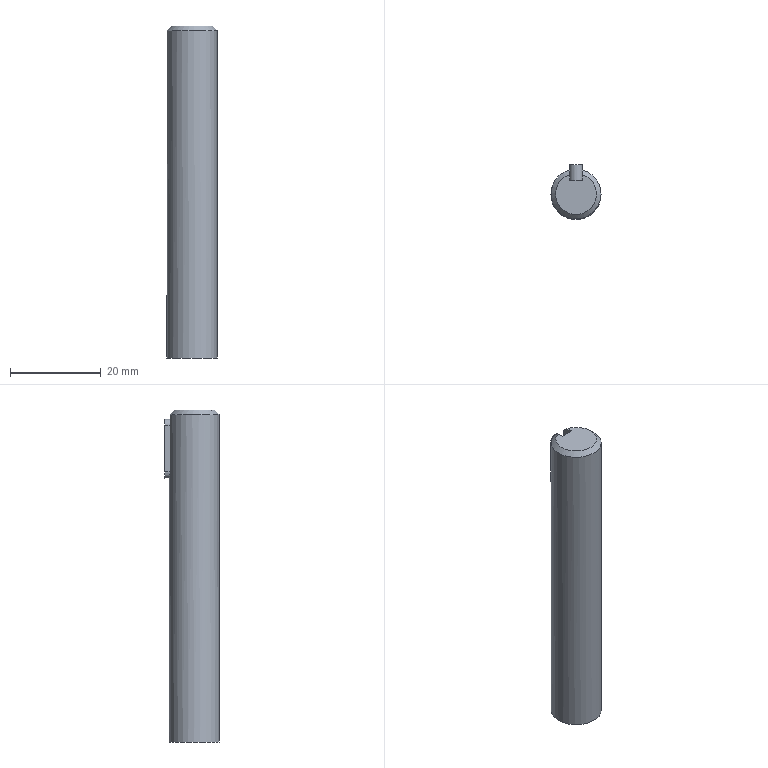Part | NX | features DATUM_CSYS 3, EXTRUDE 3, SKETCH 3, BLEND 2, BREP 1, CHAMFER 1 | 2 solids | 14 faces | box 11 x 12 x 73 mm | volume 6944 mm3 | plane 9 | cylinder 4 | cone 1 | commonest cylinder face diameters 2.8 x3 11 x1
STEP:
#1=CARTESIAN_POINT('',(-1.4,3.,69.6));
#2=VERTEX_POINT('',#1);
#3=CARTESIAN_POINT('',(-1.4,3.,59.4));
#4=VERTEX_POINT('',#3);
#5=CARTESIAN_POINT('',(-1.4,3.,71.));
#6=DIRECTION('',(0.,0.,-1.));
#7=VECTOR('',#6,1000.);
#8=LINE('',#5,#7);
#9=EDGE_CURVE('',#2,#4,#8,.T.);
#10=ORIENTED_EDGE('',*,*,#9,.F.);
#11=CARTESIAN_POINT('',(-1.4,6.5,69.6));
#12=VERTEX_POINT('',#11);
#13=CARTESIAN_POINT('',(-1.4,6.5,69.6));
#14=DIRECTION('',(0.,-1.,0.));
#15=VECTOR('',#14,1000.);
#16=LINE('',#13,#15);
#17=EDGE_CURVE('',#2,#12,#16,.F.);
#18=ORIENTED_EDGE('',*,*,#17,.T.);
#19=CARTESIAN_POINT('',(-1.4,6.5,59.4));
#20=VERTEX_POINT('',#19);
#21=CARTESIAN_POINT('',(-1.4,6.5,71.));
#22=DIRECTION('',(0.,0.,-1.));
#23=VECTOR('',#22,1000.);
#24=LINE('',#21,#23);
#25=EDGE_CURVE('',#12,#20,#24,.T.);
#26=ORIENTED_EDGE('',*,*,#25,.T.);
#27=CARTESIAN_POINT('',(-1.4,6.5,59.4));
#28=DIRECTION('',(0.,-1.,0.));
#29=VECTOR('',#28,1000.);
#30=LINE('',#27,#29);
#31=EDGE_CURVE('',#20,#4,#30,.T.);
#32=ORIENTED_EDGE('',*,*,#31,.T.);
#33=EDGE_LOOP('',(#10,#18,#26,#32));
#34=FACE_BOUND('',#33,.T.);
#35=CARTESIAN_POINT('',(-1.4,6.5,71.));
#36=DIRECTION('',(1.,0.,0.));
#37=DIRECTION('',(0.,1.,0.));
#38=AXIS2_PLACEMENT_3D('',#35,#36,#37);
#39=PLANE('',#38);
#40=ADVANCED_FACE('',(#34),#39,.F.);
#41=CARTESIAN_POINT('',(1.4,3.,69.6));
#42=VERTEX_POINT('',#41);
#43=CARTESIAN_POINT('',(0.,3.,69.6));
#44=DIRECTION('',(0.,1.,0.));
#45=DIRECTION('',(-1.,0.,0.));
#46=AXIS2_PLACEMENT_3D('',#43,#44,#45);
#47=CIRCLE('',#46,1.4);
#48=EDGE_CURVE('',#42,#2,#47,.F.);
#49=ORIENTED_EDGE('',*,*,#48,.T.);
#50=ORIENTED_EDGE('',*,*,#9,.T.);
#51=CARTESIAN_POINT('',(1.4,3.,59.4));
#52=VERTEX_POINT('',#51);
#53=CARTESIAN_POINT('',(0.,3.,59.4));
#54=DIRECTION('',(0.,1.,0.));
#55=DIRECTION('',(-1.,0.,0.));
#56=AXIS2_PLACEMENT_3D('',#53,#54,#55);
#57=CIRCLE('',#56,1.4);
#58=EDGE_CURVE('',#4,#52,#57,.F.);
#59=ORIENTED_EDGE('',*,*,#58,.T.);
#60=CARTESIAN_POINT('',(1.4,3.,71.));
#61=DIRECTION('',(0.,0.,-1.));
#62=VECTOR('',#61,1000.);
#63=LINE('',#60,#62);
#64=EDGE_CURVE('',#42,#52,#63,.T.);
#65=ORIENTED_EDGE('',*,*,#64,.F.);
#66=EDGE_LOOP('',(#49,#50,#59,#65));
#67=FACE_BOUND('',#66,.T.);
#68=CARTESIAN_POINT('',(-1.4,3.,71.));
#69=DIRECTION('',(0.,1.,0.));
#70=DIRECTION('',(-1.,0.,0.));
#71=AXIS2_PLACEMENT_3D('',#68,#69,#70);
#72=PLANE('',#71);
#73=ADVANCED_FACE('',(#67),#72,.F.);
#74=CARTESIAN_POINT('',(1.4,6.5,69.6));
#75=VERTEX_POINT('',#74);
#76=CARTESIAN_POINT('',(1.4,6.5,59.4));
#77=VERTEX_POINT('',#76);
#78=CARTESIAN_POINT('',(1.4,6.5,71.));
#79=DIRECTION('',(0.,0.,-1.));
#80=VECTOR('',#79,1000.);
#81=LINE('',#78,#80);
#82=EDGE_CURVE('',#75,#77,#81,.T.);
#83=ORIENTED_EDGE('',*,*,#82,.F.);
#84=CARTESIAN_POINT('',(1.4,3.,69.6));
#85=DIRECTION('',(0.,1.,0.));
#86=VECTOR('',#85,1000.);
#87=LINE('',#84,#86);
#88=EDGE_CURVE('',#75,#42,#87,.F.);
#89=ORIENTED_EDGE('',*,*,#88,.T.);
#90=ORIENTED_EDGE('',*,*,#64,.T.);
#91=CARTESIAN_POINT('',(1.4,3.,59.4));
#92=DIRECTION('',(0.,1.,0.));
#93=VECTOR('',#92,1000.);
#94=LINE('',#91,#93);
#95=EDGE_CURVE('',#52,#77,#94,.T.);
#96=ORIENTED_EDGE('',*,*,#95,.T.);
#97=EDGE_LOOP('',(#83,#89,#90,#96));
#98=FACE_BOUND('',#97,.T.);
#99=CARTESIAN_POINT('',(1.4,3.,71.));
#100=DIRECTION('',(-1.,0.,0.));
#101=DIRECTION('',(0.,-1.,0.));
#102=AXIS2_PLACEMENT_3D('',#99,#100,#101);
#103=PLANE('',#102);
#104=ADVANCED_FACE('',(#98),#103,.F.);
#105=ORIENTED_EDGE('',*,*,#25,.F.);
#106=CARTESIAN_POINT('',(0.,6.5,69.6));
#107=DIRECTION('',(0.,-1.,0.));
#108=DIRECTION('',(0.,0.,-1.));
#109=AXIS2_PLACEMENT_3D('',#106,#107,#108);
#110=CIRCLE('',#109,1.4);
#111=EDGE_CURVE('',#12,#75,#110,.F.);
#112=ORIENTED_EDGE('',*,*,#111,.T.);
#113=ORIENTED_EDGE('',*,*,#82,.T.);
#114=CARTESIAN_POINT('',(0.,6.5,59.4));
#115=DIRECTION('',(0.,-1.,0.));
#116=DIRECTION('',(0.,0.,-1.));
#117=AXIS2_PLACEMENT_3D('',#114,#115,#116);
#118=CIRCLE('',#117,1.4);
#119=EDGE_CURVE('',#77,#20,#118,.F.);
#120=ORIENTED_EDGE('',*,*,#119,.T.);
#121=EDGE_LOOP('',(#105,#112,#113,#120));
#122=FACE_BOUND('',#121,.T.);
#123=CARTESIAN_POINT('',(1.4,6.5,71.));
#124=DIRECTION('',(0.,-1.,0.));
#125=DIRECTION('',(0.,0.,-1.));
#126=AXIS2_PLACEMENT_3D('',#123,#124,#125);
#127=PLANE('',#126);
#128=ADVANCED_FACE('',(#122),#127,.F.);
#129=ORIENTED_EDGE('',*,*,#88,.F.);
#130=ORIENTED_EDGE('',*,*,#111,.F.);
#131=ORIENTED_EDGE('',*,*,#17,.F.);
#132=ORIENTED_EDGE('',*,*,#48,.F.);
#133=EDGE_LOOP('',(#129,#130,#131,#132));
#134=FACE_BOUND('',#133,.T.);
#135=CARTESIAN_POINT('',(0.,0.,69.6));
#136=DIRECTION('',(0.,-1.,0.));
#137=DIRECTION('',(1.,0.,0.));
#138=AXIS2_PLACEMENT_3D('',#135,#136,#137);
#139=CYLINDRICAL_SURFACE('',#138,1.4);
#140=ADVANCED_FACE('',(#134),#139,.T.);
#141=ORIENTED_EDGE('',*,*,#58,.F.);
#142=ORIENTED_EDGE('',*,*,#31,.F.);
#143=ORIENTED_EDGE('',*,*,#119,.F.);
#144=ORIENTED_EDGE('',*,*,#95,.F.);
#145=EDGE_LOOP('',(#141,#142,#143,#144));
#146=FACE_BOUND('',#145,.T.);
#147=CARTESIAN_POINT('',(0.,3.,59.4));
#148=DIRECTION('',(0.,1.,0.));
#149=DIRECTION('',(-1.,0.,0.));
#150=AXIS2_PLACEMENT_3D('',#147,#148,#149);
#151=CYLINDRICAL_SURFACE('',#150,1.4);
#152=ADVANCED_FACE('',(#146),#151,.T.);
#153=CLOSED_SHELL('',(#40,#73,#104,#128,#140,#152));
#154=MANIFOLD_SOLID_BREP('',#153);
#155=CARTESIAN_POINT('',(-1.4,4.277,73.));
#156=VERTEX_POINT('',#155);
#157=CARTESIAN_POINT('',(-1.4,3.,73.));
#158=VERTEX_POINT('',#157);
#159=CARTESIAN_POINT('',(-1.4,0.,73.));
#160=DIRECTION('',(0.,-1.,0.));
#161=VECTOR('',#160,1000.);
#162=LINE('',#159,#161);
#163=EDGE_CURVE('',#156,#158,#162,.T.);
#164=ORIENTED_EDGE('',*,*,#163,.F.);
#165=CARTESIAN_POINT('',(1.4,4.277,73.));
#166=VERTEX_POINT('',#165);
#167=CARTESIAN_POINT('',(0.,0.,73.));
#168=DIRECTION('',(0.,0.,1.));
#169=DIRECTION('',(1.,0.,0.));
#170=AXIS2_PLACEMENT_3D('',#167,#168,#169);
#171=CIRCLE('',#170,4.5);
#172=EDGE_CURVE('',#156,#166,#171,.T.);
#173=ORIENTED_EDGE('',*,*,#172,.T.);
#174=CARTESIAN_POINT('',(1.4,3.,73.));
#175=VERTEX_POINT('',#174);
#176=CARTESIAN_POINT('',(1.4,0.,73.));
#177=DIRECTION('',(0.,1.,0.));
#178=VECTOR('',#177,1000.);
#179=LINE('',#176,#178);
#180=EDGE_CURVE('',#175,#166,#179,.T.);
#181=ORIENTED_EDGE('',*,*,#180,.F.);
#182=CARTESIAN_POINT('',(0.,3.,73.));
#183=DIRECTION('',(-1.,0.,0.));
#184=VECTOR('',#183,1000.);
#185=LINE('',#182,#184);
#186=EDGE_CURVE('',#175,#158,#185,.T.);
#187=ORIENTED_EDGE('',*,*,#186,.T.);
#188=EDGE_LOOP('',(#164,#173,#181,#187));
#189=FACE_BOUND('',#188,.T.);
#190=CARTESIAN_POINT('',(0.,0.,73.));
#191=DIRECTION('',(0.,0.,1.));
#192=DIRECTION('',(1.,0.,0.));
#193=AXIS2_PLACEMENT_3D('',#190,#191,#192);
#194=PLANE('',#193);
#195=ADVANCED_FACE('',(#189),#194,.T.);
#196=CARTESIAN_POINT('',(1.4,5.319,72.));
#197=VERTEX_POINT('',#196);
#198=CARTESIAN_POINT('',(1.4,5.319,59.4));
#199=VERTEX_POINT('',#198);
#200=CARTESIAN_POINT('',(1.4,5.319,0.));
#201=DIRECTION('',(0.,0.,-1.));
#202=VECTOR('',#201,1000.);
#203=LINE('',#200,#202);
#204=EDGE_CURVE('',#197,#199,#203,.T.);
#205=ORIENTED_EDGE('',*,*,#204,.F.);
#206=CARTESIAN_POINT('',(-1.4,5.319,72.));
#207=VERTEX_POINT('',#206);
#208=CARTESIAN_POINT('',(0.,0.,72.));
#209=DIRECTION('',(0.,0.,1.));
#210=DIRECTION('',(1.,0.,0.));
#211=AXIS2_PLACEMENT_3D('',#208,#209,#210);
#212=CIRCLE('',#211,5.5);
#213=EDGE_CURVE('',#197,#207,#212,.F.);
#214=ORIENTED_EDGE('',*,*,#213,.T.);
#215=CARTESIAN_POINT('',(-1.4,5.319,59.4));
#216=VERTEX_POINT('',#215);
#217=CARTESIAN_POINT('',(-1.4,5.319,0.));
#218=DIRECTION('',(0.,0.,-1.));
#219=VECTOR('',#218,1000.);
#220=LINE('',#217,#219);
#221=EDGE_CURVE('',#216,#207,#220,.F.);
#222=ORIENTED_EDGE('',*,*,#221,.F.);
#223=CARTESIAN_POINT('',(-1.4,5.319,59.4));
#224=CARTESIAN_POINT('',(-1.4,5.319,59.029));
#225=CARTESIAN_POINT('',(-1.098,5.411,58.306));
#226=CARTESIAN_POINT('',(0.000296,5.545,57.847));
#227=CARTESIAN_POINT('',(1.097,5.411,58.305));
#228=CARTESIAN_POINT('',(1.4,5.319,59.029));
#229=CARTESIAN_POINT('',(1.4,5.319,59.4));
#230=B_SPLINE_CURVE_WITH_KNOTS('',3,(#223,#224,#225,#226,#227,#228,#229),.UNSPECIFIED.,.F.,.F.,(4,1,1,1,4),(0.,0.001098,0.002196,0.003294,0.004392),.UNSPECIFIED.);
#231=EDGE_CURVE('',#216,#199,#230,.T.);
#232=ORIENTED_EDGE('',*,*,#231,.T.);
#233=EDGE_LOOP('',(#205,#214,#222,#232));
#234=FACE_BOUND('',#233,.T.);
#235=CARTESIAN_POINT('',(-5.5,0.,0.));
#236=VERTEX_POINT('',#235);
#237=CARTESIAN_POINT('',(-5.5,0.,4.));
#238=VERTEX_POINT('',#237);
#239=CARTESIAN_POINT('',(-5.5,0.,0.));
#240=DIRECTION('',(0.,0.,-1.));
#241=VECTOR('',#240,1000.);
#242=LINE('',#239,#241);
#243=EDGE_CURVE('',#236,#238,#242,.F.);
#244=ORIENTED_EDGE('',*,*,#243,.T.);
#245=ORIENTED_EDGE('',*,*,#243,.F.);
#246=CARTESIAN_POINT('',(5.5,0.,0.));
#247=VERTEX_POINT('',#246);
#248=CARTESIAN_POINT('',(0.,0.,0.));
#249=DIRECTION('',(0.,0.,-1.));
#250=DIRECTION('',(-1.,0.,0.));
#251=AXIS2_PLACEMENT_3D('',#248,#249,#250);
#252=CIRCLE('',#251,5.5);
#253=EDGE_CURVE('',#247,#236,#252,.T.);
#254=ORIENTED_EDGE('',*,*,#253,.F.);
#255=CARTESIAN_POINT('',(5.5,0.,4.));
#256=VERTEX_POINT('',#255);
#257=CARTESIAN_POINT('',(5.5,0.,0.));
#258=DIRECTION('',(0.,0.,-1.));
#259=VECTOR('',#258,1000.);
#260=LINE('',#257,#259);
#261=EDGE_CURVE('',#247,#256,#260,.F.);
#262=ORIENTED_EDGE('',*,*,#261,.T.);
#263=ORIENTED_EDGE('',*,*,#261,.F.);
#264=CARTESIAN_POINT('',(0.,0.,0.));
#265=DIRECTION('',(0.,0.,-1.));
#266=DIRECTION('',(-1.,0.,0.));
#267=AXIS2_PLACEMENT_3D('',#264,#265,#266);
#268=CIRCLE('',#267,5.5);
#269=EDGE_CURVE('',#236,#247,#268,.T.);
#270=ORIENTED_EDGE('',*,*,#269,.F.);
#271=EDGE_LOOP('',(#244,#245,#254,#262,#263,#270));
#272=FACE_BOUND('',#271,.T.);
#273=CARTESIAN_POINT('',(0.,0.,0.));
#274=DIRECTION('',(0.,0.,-1.));
#275=DIRECTION('',(1.,0.,0.));
#276=AXIS2_PLACEMENT_3D('',#273,#274,#275);
#277=CYLINDRICAL_SURFACE('',#276,5.5);
#278=ADVANCED_FACE('',(#234,#272),#277,.T.);
#279=ORIENTED_EDGE('',*,*,#269,.T.);
#280=ORIENTED_EDGE('',*,*,#253,.T.);
#281=EDGE_LOOP('',(#279,#280));
#282=FACE_BOUND('',#281,.T.);
#283=CARTESIAN_POINT('',(0.,5.5,0.));
#284=DIRECTION('',(0.,0.,-1.));
#285=DIRECTION('',(1.,0.,0.));
#286=AXIS2_PLACEMENT_3D('',#283,#284,#285);
#287=PLANE('',#286);
#288=ADVANCED_FACE('',(#282),#287,.T.);
#289=ORIENTED_EDGE('',*,*,#221,.T.);
#290=CARTESIAN_POINT('',(-1.4,5.319,72.));
#291=CARTESIAN_POINT('',(-1.4,4.973,72.335));
#292=CARTESIAN_POINT('',(-1.4,4.626,72.668));
#293=CARTESIAN_POINT('',(-1.4,4.277,73.));
#294=B_SPLINE_CURVE_WITH_KNOTS('',3,(#290,#291,#292,#293),.UNSPECIFIED.,.F.,.F.,(4,4),(0.,0.001444),.UNSPECIFIED.);
#295=EDGE_CURVE('',#207,#156,#294,.T.);
#296=ORIENTED_EDGE('',*,*,#295,.T.);
#297=ORIENTED_EDGE('',*,*,#163,.T.);
#298=CARTESIAN_POINT('',(-1.4,3.,59.4));
#299=VERTEX_POINT('',#298);
#300=CARTESIAN_POINT('',(-1.4,3.,58.));
#301=DIRECTION('',(0.,0.,1.));
#302=VECTOR('',#301,1000.);
#303=LINE('',#300,#302);
#304=EDGE_CURVE('',#158,#299,#303,.F.);
#305=ORIENTED_EDGE('',*,*,#304,.T.);
#306=CARTESIAN_POINT('',(-1.4,5.319,59.4));
#307=DIRECTION('',(0.,-1.,0.));
#308=VECTOR('',#307,1000.);
#309=LINE('',#306,#308);
#310=EDGE_CURVE('',#299,#216,#309,.F.);
#311=ORIENTED_EDGE('',*,*,#310,.T.);
#312=EDGE_LOOP('',(#289,#296,#297,#305,#311));
#313=FACE_BOUND('',#312,.T.);
#314=CARTESIAN_POINT('',(-1.4,3.,58.));
#315=DIRECTION('',(-1.,0.,0.));
#316=DIRECTION('',(0.,0.,1.));
#317=AXIS2_PLACEMENT_3D('',#314,#315,#316);
#318=PLANE('',#317);
#319=ADVANCED_FACE('',(#313),#318,.F.);
#320=ORIENTED_EDGE('',*,*,#180,.T.);
#321=CARTESIAN_POINT('',(1.4,4.277,73.));
#322=CARTESIAN_POINT('',(1.4,4.626,72.668));
#323=CARTESIAN_POINT('',(1.4,4.973,72.335));
#324=CARTESIAN_POINT('',(1.4,5.319,72.));
#325=B_SPLINE_CURVE_WITH_KNOTS('',3,(#321,#322,#323,#324),.UNSPECIFIED.,.F.,.F.,(4,4),(0.,0.001444),.UNSPECIFIED.);
#326=EDGE_CURVE('',#166,#197,#325,.T.);
#327=ORIENTED_EDGE('',*,*,#326,.T.);
#328=ORIENTED_EDGE('',*,*,#204,.T.);
#329=CARTESIAN_POINT('',(1.4,3.,59.4));
#330=VERTEX_POINT('',#329);
#331=CARTESIAN_POINT('',(1.4,3.,59.4));
#332=DIRECTION('',(0.,-1.,0.));
#333=VECTOR('',#332,1000.);
#334=LINE('',#331,#333);
#335=EDGE_CURVE('',#199,#330,#334,.T.);
#336=ORIENTED_EDGE('',*,*,#335,.T.);
#337=CARTESIAN_POINT('',(1.4,3.,78.));
#338=DIRECTION('',(0.,0.,-1.));
#339=VECTOR('',#338,1000.);
#340=LINE('',#337,#339);
#341=EDGE_CURVE('',#330,#175,#340,.F.);
#342=ORIENTED_EDGE('',*,*,#341,.T.);
#343=EDGE_LOOP('',(#320,#327,#328,#336,#342));
#344=FACE_BOUND('',#343,.T.);
#345=CARTESIAN_POINT('',(1.4,3.,78.));
#346=DIRECTION('',(1.,0.,0.));
#347=DIRECTION('',(0.,0.,-1.));
#348=AXIS2_PLACEMENT_3D('',#345,#346,#347);
#349=PLANE('',#348);
#350=ADVANCED_FACE('',(#344),#349,.F.);
#351=CARTESIAN_POINT('',(0.,3.,59.4));
#352=DIRECTION('',(0.,1.,0.));
#353=DIRECTION('',(0.,0.,1.));
#354=AXIS2_PLACEMENT_3D('',#351,#352,#353);
#355=CIRCLE('',#354,1.4);
#356=EDGE_CURVE('',#330,#299,#355,.T.);
#357=ORIENTED_EDGE('',*,*,#356,.T.);
#358=ORIENTED_EDGE('',*,*,#304,.F.);
#359=ORIENTED_EDGE('',*,*,#186,.F.);
#360=ORIENTED_EDGE('',*,*,#341,.F.);
#361=EDGE_LOOP('',(#357,#358,#359,#360));
#362=FACE_BOUND('',#361,.T.);
#363=CARTESIAN_POINT('',(0.,3.,0.));
#364=DIRECTION('',(0.,1.,0.));
#365=DIRECTION('',(0.,0.,1.));
#366=AXIS2_PLACEMENT_3D('',#363,#364,#365);
#367=PLANE('',#366);
#368=ADVANCED_FACE('',(#362),#367,.T.);
#369=ORIENTED_EDGE('',*,*,#335,.F.);
#370=ORIENTED_EDGE('',*,*,#231,.F.);
#371=ORIENTED_EDGE('',*,*,#310,.F.);
#372=ORIENTED_EDGE('',*,*,#356,.F.);
#373=EDGE_LOOP('',(#369,#370,#371,#372));
#374=FACE_BOUND('',#373,.T.);
#375=CARTESIAN_POINT('',(0.,3.,59.4));
#376=DIRECTION('',(0.,1.,0.));
#377=DIRECTION('',(0.,0.,1.));
#378=AXIS2_PLACEMENT_3D('',#375,#376,#377);
#379=CYLINDRICAL_SURFACE('',#378,1.4);
#380=ADVANCED_FACE('',(#374),#379,.F.);
#381=ORIENTED_EDGE('',*,*,#295,.F.);
#382=ORIENTED_EDGE('',*,*,#213,.F.);
#383=ORIENTED_EDGE('',*,*,#326,.F.);
#384=ORIENTED_EDGE('',*,*,#172,.F.);
#385=EDGE_LOOP('',(#381,#382,#383,#384));
#386=FACE_BOUND('',#385,.T.);
#387=CARTESIAN_POINT('',(0.,0.,73.));
#388=DIRECTION('',(0.,0.,-1.));
#389=DIRECTION('',(-1.,0.,0.));
#390=AXIS2_PLACEMENT_3D('',#387,#388,#389);
#391=CONICAL_SURFACE('',#390,4.5,0.7854);
#392=ADVANCED_FACE('',(#386),#391,.T.);
#393=CLOSED_SHELL('',(#195,#278,#288,#319,#350,#368,#380,#392));
#394=MANIFOLD_SOLID_BREP('',#393);
#395=(LENGTH_UNIT()NAMED_UNIT(*)SI_UNIT(.MILLI.,.METRE.));
#396=UNCERTAINTY_MEASURE_WITH_UNIT(LENGTH_MEASURE(0.0508),#395,'','');
#397=(NAMED_UNIT(*)PLANE_ANGLE_UNIT()SI_UNIT($,.RADIAN.));
#398=(NAMED_UNIT(*)SI_UNIT($,.STERADIAN.)SOLID_ANGLE_UNIT());
#399=(GEOMETRIC_REPRESENTATION_CONTEXT(3)GLOBAL_UNCERTAINTY_ASSIGNED_CONTEXT((#396))GLOBAL_UNIT_ASSIGNED_CONTEXT((#395,#397,#398))REPRESENTATION_CONTEXT('',''));
#400=ADVANCED_BREP_SHAPE_REPRESENTATION('',(#154,#394),#399);